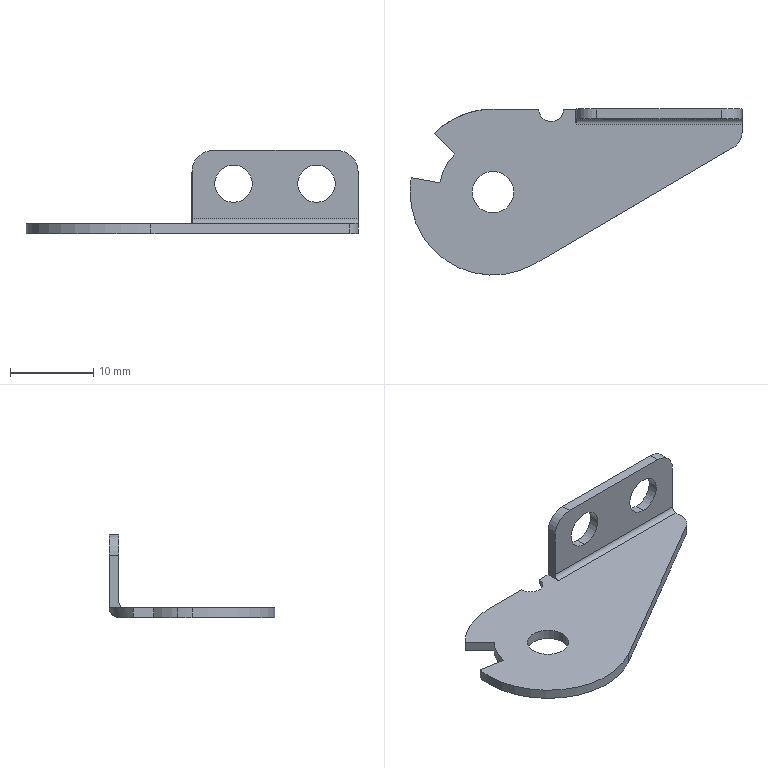Part | STEP file | 1 solid | 27 faces | box 40 x 20 x 10 mm | volume 758.925 mm3 | cylinder 17 | plane 10 | commonest cylinder face diameters 4.5 x4 5 x4 20 x3 2.4 x2 1.2 x1 3 x1